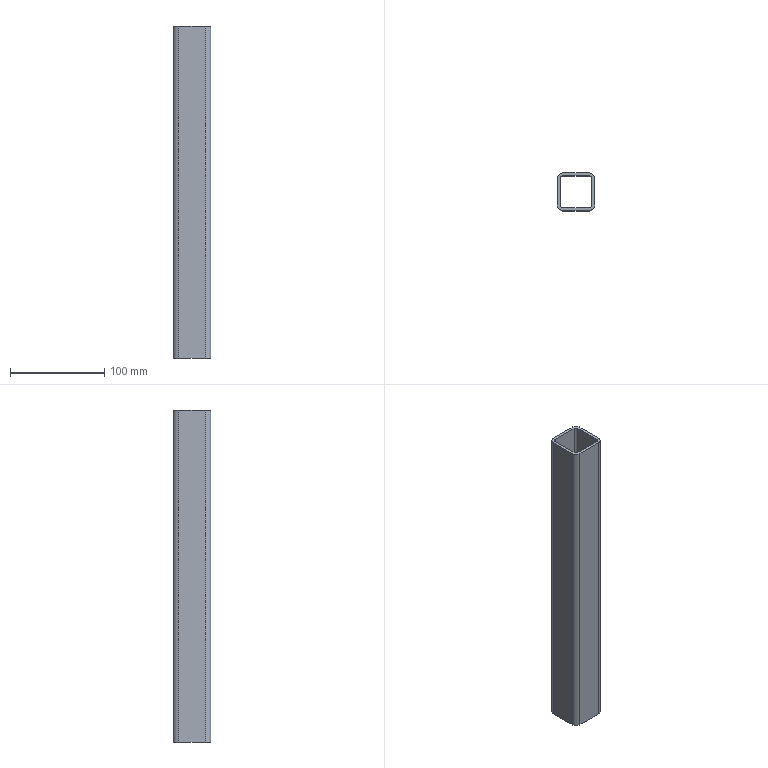Part | STEP file | SN10_003_008-09_TUBO_QUADRADO | 1 solid | 18 faces | box 40 x 40 x 353 mm | volume 148551 mm3 | plane 10 | cylinder 8 | commonest cylinder face diameters 6 x4 12 x4
STEP:
#1=CARTESIAN_POINT('',(0.,0.,0.));
#2=DIRECTION('',(0.,0.,1.));
#3=DIRECTION('',(1.,0.,0.));
#4=AXIS2_PLACEMENT_3D('',#1,#2,#3);
#5=CARTESIAN_POINT('',(3482.,140.,-373.));
#6=VERTEX_POINT('',#5);
#7=CARTESIAN_POINT('',(3488.,146.,-373.));
#8=VERTEX_POINT('',#7);
#9=CARTESIAN_POINT('',(3482.,146.,-373.));
#10=DIRECTION('',(0.,0.,1.));
#11=DIRECTION('',(1.,0.,0.));
#12=AXIS2_PLACEMENT_3D('',#9,#10,#11);
#13=CIRCLE('',#12,6.);
#14=CARTESIAN_POINT('',(3482.,146.,-196.5));
#15=DIRECTION('',(0.,0.,1.));
#16=DIRECTION('',(0.,-1.,0.));
#17=AXIS2_PLACEMENT_3D('',#14,#15,#16);
#18=CYLINDRICAL_SURFACE('',#17,6.);
#19=CARTESIAN_POINT('',(-4.712,-176.5));
#20=DIRECTION('',(1.,0.));
#21=VECTOR('',#20,1.);
#22=LINE('',#19,#21);
#23=(GEOMETRIC_REPRESENTATION_CONTEXT(2)PARAMETRIC_REPRESENTATION_CONTEXT()REPRESENTATION_CONTEXT('',''));
#24=DEFINITIONAL_REPRESENTATION('',(#22),#23);
#25=PCURVE('',#18,#24);
#26=CARTESIAN_POINT('',(0.,0.,-373.));
#27=DIRECTION('',(0.,0.,1.));
#28=DIRECTION('',(1.,0.,0.));
#29=AXIS2_PLACEMENT_3D('',#26,#27,#28);
#30=PLANE('',#29);
#31=CARTESIAN_POINT('',(3482.,146.));
#32=DIRECTION('',(1.,0.));
#33=AXIS2_PLACEMENT_2D('',#31,#32);
#34=CIRCLE('',#33,6.);
#35=(GEOMETRIC_REPRESENTATION_CONTEXT(2)PARAMETRIC_REPRESENTATION_CONTEXT()REPRESENTATION_CONTEXT('',''));
#36=DEFINITIONAL_REPRESENTATION('',(#34),#35);
#37=PCURVE('',#30,#36);
#38=SURFACE_CURVE('',#13,(#25,#37),.PCURVE_S1.);
#39=EDGE_CURVE('',#6,#8,#38,.T.);
#40=ORIENTED_EDGE('',*,*,#39,.T.);
#41=CARTESIAN_POINT('',(3488.,146.,-20.));
#42=VERTEX_POINT('',#41);
#43=CARTESIAN_POINT('',(3488.,146.,-373.));
#44=DIRECTION('',(0.,0.,1.));
#45=VECTOR('',#44,1.);
#46=LINE('',#43,#45);
#47=CARTESIAN_POINT('',(1.571,-176.5));
#48=DIRECTION('',(0.,1.));
#49=VECTOR('',#48,1.);
#50=LINE('',#47,#49);
#51=(GEOMETRIC_REPRESENTATION_CONTEXT(2)PARAMETRIC_REPRESENTATION_CONTEXT()REPRESENTATION_CONTEXT('',''));
#52=DEFINITIONAL_REPRESENTATION('',(#50),#51);
#53=PCURVE('',#18,#52);
#54=CARTESIAN_POINT('',(3488.,146.,-20.));
#55=DIRECTION('',(-1.,0.,0.));
#56=DIRECTION('',(0.,0.,1.));
#57=AXIS2_PLACEMENT_3D('',#54,#55,#56);
#58=PLANE('',#57);
#59=CARTESIAN_POINT('',(-353.,0.));
#60=DIRECTION('',(1.,0.));
#61=VECTOR('',#60,1.);
#62=LINE('',#59,#61);
#63=(GEOMETRIC_REPRESENTATION_CONTEXT(2)PARAMETRIC_REPRESENTATION_CONTEXT()REPRESENTATION_CONTEXT('',''));
#64=DEFINITIONAL_REPRESENTATION('',(#62),#63);
#65=PCURVE('',#58,#64);
#66=SURFACE_CURVE('',#46,(#53,#65),.PCURVE_S1.);
#67=EDGE_CURVE('',#8,#42,#66,.T.);
#68=ORIENTED_EDGE('',*,*,#67,.T.);
#69=CARTESIAN_POINT('',(3482.,140.,-20.));
#70=VERTEX_POINT('',#69);
#71=CARTESIAN_POINT('',(3482.,146.,-20.));
#72=DIRECTION('',(0.,0.,1.));
#73=DIRECTION('',(1.,0.,0.));
#74=AXIS2_PLACEMENT_3D('',#71,#72,#73);
#75=CIRCLE('',#74,6.);
#76=CARTESIAN_POINT('',(-4.712,176.5));
#77=DIRECTION('',(1.,0.));
#78=VECTOR('',#77,1.);
#79=LINE('',#76,#78);
#80=(GEOMETRIC_REPRESENTATION_CONTEXT(2)PARAMETRIC_REPRESENTATION_CONTEXT()REPRESENTATION_CONTEXT('',''));
#81=DEFINITIONAL_REPRESENTATION('',(#79),#80);
#82=PCURVE('',#18,#81);
#83=CARTESIAN_POINT('',(0.,0.,-20.));
#84=DIRECTION('',(0.,0.,1.));
#85=DIRECTION('',(1.,0.,0.));
#86=AXIS2_PLACEMENT_3D('',#83,#84,#85);
#87=PLANE('',#86);
#88=CARTESIAN_POINT('',(3482.,146.));
#89=DIRECTION('',(1.,0.));
#90=AXIS2_PLACEMENT_2D('',#88,#89);
#91=CIRCLE('',#90,6.);
#92=(GEOMETRIC_REPRESENTATION_CONTEXT(2)PARAMETRIC_REPRESENTATION_CONTEXT()REPRESENTATION_CONTEXT('',''));
#93=DEFINITIONAL_REPRESENTATION('',(#91),#92);
#94=PCURVE('',#87,#93);
#95=SURFACE_CURVE('',#75,(#82,#94),.PCURVE_S1.);
#96=EDGE_CURVE('',#70,#42,#95,.T.);
#97=ORIENTED_EDGE('',*,*,#96,.F.);
#98=CARTESIAN_POINT('',(3482.,140.,-373.));
#99=DIRECTION('',(0.,0.,1.));
#100=VECTOR('',#99,1.);
#101=LINE('',#98,#100);
#102=CARTESIAN_POINT('',(0.,-176.5));
#103=DIRECTION('',(0.,1.));
#104=VECTOR('',#103,1.);
#105=LINE('',#102,#104);
#106=(GEOMETRIC_REPRESENTATION_CONTEXT(2)PARAMETRIC_REPRESENTATION_CONTEXT()REPRESENTATION_CONTEXT('',''));
#107=DEFINITIONAL_REPRESENTATION('',(#105),#106);
#108=PCURVE('',#18,#107);
#109=CARTESIAN_POINT('',(3454.,140.,-20.));
#110=DIRECTION('',(0.,1.,0.));
#111=DIRECTION('',(0.,0.,1.));
#112=AXIS2_PLACEMENT_3D('',#109,#110,#111);
#113=PLANE('',#112);
#114=CARTESIAN_POINT('',(-353.,28.));
#115=DIRECTION('',(1.,0.));
#116=VECTOR('',#115,1.);
#117=LINE('',#114,#116);
#118=(GEOMETRIC_REPRESENTATION_CONTEXT(2)PARAMETRIC_REPRESENTATION_CONTEXT()REPRESENTATION_CONTEXT('',''));
#119=DEFINITIONAL_REPRESENTATION('',(#117),#118);
#120=PCURVE('',#113,#119);
#121=SURFACE_CURVE('',#101,(#108,#120),.PCURVE_S1.);
#122=EDGE_CURVE('',#6,#70,#121,.T.);
#123=ORIENTED_EDGE('',*,*,#122,.F.);
#124=EDGE_LOOP('',(#40,#68,#97,#123));
#125=FACE_BOUND('',#124,.T.);
#126=ADVANCED_FACE('',(#125),#18,.T.);
#127=CARTESIAN_POINT('',(3488.,174.,-373.));
#128=VERTEX_POINT('',#127);
#129=CARTESIAN_POINT('',(3488.,146.,-373.));
#130=DIRECTION('',(0.,1.,0.));
#131=VECTOR('',#130,1.);
#132=LINE('',#129,#131);
#133=CARTESIAN_POINT('',(-353.,0.));
#134=DIRECTION('',(0.,1.));
#135=VECTOR('',#134,1.);
#136=LINE('',#133,#135);
#137=(GEOMETRIC_REPRESENTATION_CONTEXT(2)PARAMETRIC_REPRESENTATION_CONTEXT()REPRESENTATION_CONTEXT('',''));
#138=DEFINITIONAL_REPRESENTATION('',(#136),#137);
#139=PCURVE('',#58,#138);
#140=CARTESIAN_POINT('',(3488.,146.));
#141=DIRECTION('',(0.,1.));
#142=VECTOR('',#141,1.);
#143=LINE('',#140,#142);
#144=(GEOMETRIC_REPRESENTATION_CONTEXT(2)PARAMETRIC_REPRESENTATION_CONTEXT()REPRESENTATION_CONTEXT('',''));
#145=DEFINITIONAL_REPRESENTATION('',(#143),#144);
#146=PCURVE('',#30,#145);
#147=SURFACE_CURVE('',#132,(#139,#146),.PCURVE_S1.);
#148=EDGE_CURVE('',#8,#128,#147,.T.);
#149=ORIENTED_EDGE('',*,*,#148,.T.);
#150=CARTESIAN_POINT('',(3488.,174.,-20.));
#151=VERTEX_POINT('',#150);
#152=CARTESIAN_POINT('',(3488.,174.,-20.));
#153=DIRECTION('',(0.,0.,-1.));
#154=VECTOR('',#153,1.);
#155=LINE('',#152,#154);
#156=CARTESIAN_POINT('',(0.,28.));
#157=DIRECTION('',(-1.,0.));
#158=VECTOR('',#157,1.);
#159=LINE('',#156,#158);
#160=(GEOMETRIC_REPRESENTATION_CONTEXT(2)PARAMETRIC_REPRESENTATION_CONTEXT()REPRESENTATION_CONTEXT('',''));
#161=DEFINITIONAL_REPRESENTATION('',(#159),#160);
#162=PCURVE('',#58,#161);
#163=CARTESIAN_POINT('',(3482.,174.,-196.5));
#164=DIRECTION('',(0.,0.,1.));
#165=DIRECTION('',(1.,0.,0.));
#166=AXIS2_PLACEMENT_3D('',#163,#164,#165);
#167=CYLINDRICAL_SURFACE('',#166,6.);
#168=CARTESIAN_POINT('',(0.,176.5));
#169=DIRECTION('',(0.,-1.));
#170=VECTOR('',#169,1.);
#171=LINE('',#168,#170);
#172=(GEOMETRIC_REPRESENTATION_CONTEXT(2)PARAMETRIC_REPRESENTATION_CONTEXT()REPRESENTATION_CONTEXT('',''));
#173=DEFINITIONAL_REPRESENTATION('',(#171),#172);
#174=PCURVE('',#167,#173);
#175=SURFACE_CURVE('',#155,(#162,#174),.PCURVE_S1.);
#176=EDGE_CURVE('',#151,#128,#175,.T.);
#177=ORIENTED_EDGE('',*,*,#176,.F.);
#178=CARTESIAN_POINT('',(3488.,146.,-20.));
#179=DIRECTION('',(0.,1.,0.));
#180=VECTOR('',#179,1.);
#181=LINE('',#178,#180);
#182=CARTESIAN_POINT('',(0.,0.));
#183=DIRECTION('',(0.,1.));
#184=VECTOR('',#183,1.);
#185=LINE('',#182,#184);
#186=(GEOMETRIC_REPRESENTATION_CONTEXT(2)PARAMETRIC_REPRESENTATION_CONTEXT()REPRESENTATION_CONTEXT('',''));
#187=DEFINITIONAL_REPRESENTATION('',(#185),#186);
#188=PCURVE('',#58,#187);
#189=CARTESIAN_POINT('',(3488.,146.));
#190=DIRECTION('',(0.,1.));
#191=VECTOR('',#190,1.);
#192=LINE('',#189,#191);
#193=(GEOMETRIC_REPRESENTATION_CONTEXT(2)PARAMETRIC_REPRESENTATION_CONTEXT()REPRESENTATION_CONTEXT('',''));
#194=DEFINITIONAL_REPRESENTATION('',(#192),#193);
#195=PCURVE('',#87,#194);
#196=SURFACE_CURVE('',#181,(#188,#195),.PCURVE_S1.);
#197=EDGE_CURVE('',#42,#151,#196,.T.);
#198=ORIENTED_EDGE('',*,*,#197,.F.);
#199=ORIENTED_EDGE('',*,*,#67,.F.);
#200=EDGE_LOOP('',(#149,#177,#198,#199));
#201=FACE_BOUND('',#200,.T.);
#202=ADVANCED_FACE('',(#201),#58,.F.);
#203=CARTESIAN_POINT('',(3482.,180.,-373.));
#204=VERTEX_POINT('',#203);
#205=CARTESIAN_POINT('',(3482.,174.,-373.));
#206=DIRECTION('',(0.,0.,1.));
#207=DIRECTION('',(1.,0.,0.));
#208=AXIS2_PLACEMENT_3D('',#205,#206,#207);
#209=CIRCLE('',#208,6.);
#210=CARTESIAN_POINT('',(0.,-176.5));
#211=DIRECTION('',(1.,0.));
#212=VECTOR('',#211,1.);
#213=LINE('',#210,#212);
#214=(GEOMETRIC_REPRESENTATION_CONTEXT(2)PARAMETRIC_REPRESENTATION_CONTEXT()REPRESENTATION_CONTEXT('',''));
#215=DEFINITIONAL_REPRESENTATION('',(#213),#214);
#216=PCURVE('',#167,#215);
#217=CARTESIAN_POINT('',(3482.,174.));
#218=DIRECTION('',(1.,0.));
#219=AXIS2_PLACEMENT_2D('',#217,#218);
#220=CIRCLE('',#219,6.);
#221=(GEOMETRIC_REPRESENTATION_CONTEXT(2)PARAMETRIC_REPRESENTATION_CONTEXT()REPRESENTATION_CONTEXT('',''));
#222=DEFINITIONAL_REPRESENTATION('',(#220),#221);
#223=PCURVE('',#30,#222);
#224=SURFACE_CURVE('',#209,(#216,#223),.PCURVE_S1.);
#225=EDGE_CURVE('',#128,#204,#224,.T.);
#226=ORIENTED_EDGE('',*,*,#225,.T.);
#227=CARTESIAN_POINT('',(3482.,180.,-20.));
#228=VERTEX_POINT('',#227);
#229=CARTESIAN_POINT('',(3482.,180.,-373.));
#230=DIRECTION('',(0.,0.,1.));
#231=VECTOR('',#230,1.);
#232=LINE('',#229,#231);
#233=CARTESIAN_POINT('',(1.571,-176.5));
#234=DIRECTION('',(0.,1.));
#235=VECTOR('',#234,1.);
#236=LINE('',#233,#235);
#237=(GEOMETRIC_REPRESENTATION_CONTEXT(2)PARAMETRIC_REPRESENTATION_CONTEXT()REPRESENTATION_CONTEXT('',''));
#238=DEFINITIONAL_REPRESENTATION('',(#236),#237);
#239=PCURVE('',#167,#238);
#240=CARTESIAN_POINT('',(3482.,180.,-20.));
#241=DIRECTION('',(0.,-1.,0.));
#242=DIRECTION('',(0.,0.,-1.));
#243=AXIS2_PLACEMENT_3D('',#240,#241,#242);
#244=PLANE('',#243);
#245=CARTESIAN_POINT('',(353.,0.));
#246=DIRECTION('',(-1.,0.));
#247=VECTOR('',#246,1.);
#248=LINE('',#245,#247);
#249=(GEOMETRIC_REPRESENTATION_CONTEXT(2)PARAMETRIC_REPRESENTATION_CONTEXT()REPRESENTATION_CONTEXT('',''));
#250=DEFINITIONAL_REPRESENTATION('',(#248),#249);
#251=PCURVE('',#244,#250);
#252=SURFACE_CURVE('',#232,(#239,#251),.PCURVE_S1.);
#253=EDGE_CURVE('',#204,#228,#252,.T.);
#254=ORIENTED_EDGE('',*,*,#253,.T.);
#255=CARTESIAN_POINT('',(3482.,174.,-20.));
#256=DIRECTION('',(0.,0.,1.));
#257=DIRECTION('',(1.,0.,0.));
#258=AXIS2_PLACEMENT_3D('',#255,#256,#257);
#259=CIRCLE('',#258,6.);
#260=CARTESIAN_POINT('',(0.,176.5));
#261=DIRECTION('',(1.,0.));
#262=VECTOR('',#261,1.);
#263=LINE('',#260,#262);
#264=(GEOMETRIC_REPRESENTATION_CONTEXT(2)PARAMETRIC_REPRESENTATION_CONTEXT()REPRESENTATION_CONTEXT('',''));
#265=DEFINITIONAL_REPRESENTATION('',(#263),#264);
#266=PCURVE('',#167,#265);
#267=CARTESIAN_POINT('',(3482.,174.));
#268=DIRECTION('',(1.,0.));
#269=AXIS2_PLACEMENT_2D('',#267,#268);
#270=CIRCLE('',#269,6.);
#271=(GEOMETRIC_REPRESENTATION_CONTEXT(2)PARAMETRIC_REPRESENTATION_CONTEXT()REPRESENTATION_CONTEXT('',''));
#272=DEFINITIONAL_REPRESENTATION('',(#270),#271);
#273=PCURVE('',#87,#272);
#274=SURFACE_CURVE('',#259,(#266,#273),.PCURVE_S1.);
#275=EDGE_CURVE('',#151,#228,#274,.T.);
#276=ORIENTED_EDGE('',*,*,#275,.F.);
#277=ORIENTED_EDGE('',*,*,#176,.T.);
#278=EDGE_LOOP('',(#226,#254,#276,#277));
#279=FACE_BOUND('',#278,.T.);
#280=ADVANCED_FACE('',(#279),#167,.T.);
#281=CARTESIAN_POINT('',(3454.,180.,-373.));
#282=VERTEX_POINT('',#281);
#283=CARTESIAN_POINT('',(3482.,180.,-373.));
#284=DIRECTION('',(-1.,0.,0.));
#285=VECTOR('',#284,1.);
#286=LINE('',#283,#285);
#287=CARTESIAN_POINT('',(353.,0.));
#288=DIRECTION('',(0.,-1.));
#289=VECTOR('',#288,1.);
#290=LINE('',#287,#289);
#291=(GEOMETRIC_REPRESENTATION_CONTEXT(2)PARAMETRIC_REPRESENTATION_CONTEXT()REPRESENTATION_CONTEXT('',''));
#292=DEFINITIONAL_REPRESENTATION('',(#290),#291);
#293=PCURVE('',#244,#292);
#294=CARTESIAN_POINT('',(3482.,180.));
#295=DIRECTION('',(-1.,0.));
#296=VECTOR('',#295,1.);
#297=LINE('',#294,#296);
#298=(GEOMETRIC_REPRESENTATION_CONTEXT(2)PARAMETRIC_REPRESENTATION_CONTEXT()REPRESENTATION_CONTEXT('',''));
#299=DEFINITIONAL_REPRESENTATION('',(#297),#298);
#300=PCURVE('',#30,#299);
#301=SURFACE_CURVE('',#286,(#293,#300),.PCURVE_S1.);
#302=EDGE_CURVE('',#204,#282,#301,.T.);
#303=ORIENTED_EDGE('',*,*,#302,.T.);
#304=CARTESIAN_POINT('',(3454.,180.,-20.));
#305=VERTEX_POINT('',#304);
#306=CARTESIAN_POINT('',(3454.,180.,-20.));
#307=DIRECTION('',(0.,0.,-1.));
#308=VECTOR('',#307,1.);
#309=LINE('',#306,#308);
#310=CARTESIAN_POINT('',(0.,-28.));
#311=DIRECTION('',(1.,0.));
#312=VECTOR('',#311,1.);
#313=LINE('',#310,#312);
#314=(GEOMETRIC_REPRESENTATION_CONTEXT(2)PARAMETRIC_REPRESENTATION_CONTEXT()REPRESENTATION_CONTEXT('',''));
#315=DEFINITIONAL_REPRESENTATION('',(#313),#314);
#316=PCURVE('',#244,#315);
#317=CARTESIAN_POINT('',(3454.,174.,-196.5));
#318=DIRECTION('',(0.,0.,1.));
#319=DIRECTION('',(0.,1.,0.));
#320=AXIS2_PLACEMENT_3D('',#317,#318,#319);
#321=CYLINDRICAL_SURFACE('',#320,6.);
#322=CARTESIAN_POINT('',(0.,176.5));
#323=DIRECTION('',(0.,-1.));
#324=VECTOR('',#323,1.);
#325=LINE('',#322,#324);
#326=(GEOMETRIC_REPRESENTATION_CONTEXT(2)PARAMETRIC_REPRESENTATION_CONTEXT()REPRESENTATION_CONTEXT('',''));
#327=DEFINITIONAL_REPRESENTATION('',(#325),#326);
#328=PCURVE('',#321,#327);
#329=SURFACE_CURVE('',#309,(#316,#328),.PCURVE_S1.);
#330=EDGE_CURVE('',#305,#282,#329,.T.);
#331=ORIENTED_EDGE('',*,*,#330,.F.);
#332=CARTESIAN_POINT('',(3482.,180.,-20.));
#333=DIRECTION('',(-1.,0.,0.));
#334=VECTOR('',#333,1.);
#335=LINE('',#332,#334);
#336=CARTESIAN_POINT('',(0.,0.));
#337=DIRECTION('',(0.,-1.));
#338=VECTOR('',#337,1.);
#339=LINE('',#336,#338);
#340=(GEOMETRIC_REPRESENTATION_CONTEXT(2)PARAMETRIC_REPRESENTATION_CONTEXT()REPRESENTATION_CONTEXT('',''));
#341=DEFINITIONAL_REPRESENTATION('',(#339),#340);
#342=PCURVE('',#244,#341);
#343=CARTESIAN_POINT('',(3482.,180.));
#344=DIRECTION('',(-1.,0.));
#345=VECTOR('',#344,1.);
#346=LINE('',#343,#345);
#347=(GEOMETRIC_REPRESENTATION_CONTEXT(2)PARAMETRIC_REPRESENTATION_CONTEXT()REPRESENTATION_CONTEXT('',''));
#348=DEFINITIONAL_REPRESENTATION('',(#346),#347);
#349=PCURVE('',#87,#348);
#350=SURFACE_CURVE('',#335,(#342,#349),.PCURVE_S1.);
#351=EDGE_CURVE('',#228,#305,#350,.T.);
#352=ORIENTED_EDGE('',*,*,#351,.F.);
#353=ORIENTED_EDGE('',*,*,#253,.F.);
#354=EDGE_LOOP('',(#303,#331,#352,#353));
#355=FACE_BOUND('',#354,.T.);
#356=ADVANCED_FACE('',(#355),#244,.F.);
#357=CARTESIAN_POINT('',(3448.,174.,-373.));
#358=VERTEX_POINT('',#357);
#359=CARTESIAN_POINT('',(3454.,174.,-373.));
#360=DIRECTION('',(0.,0.,1.));
#361=DIRECTION('',(1.,0.,0.));
#362=AXIS2_PLACEMENT_3D('',#359,#360,#361);
#363=CIRCLE('',#362,6.);
#364=CARTESIAN_POINT('',(-1.571,-176.5));
#365=DIRECTION('',(1.,0.));
#366=VECTOR('',#365,1.);
#367=LINE('',#364,#366);
#368=(GEOMETRIC_REPRESENTATION_CONTEXT(2)PARAMETRIC_REPRESENTATION_CONTEXT()REPRESENTATION_CONTEXT('',''));
#369=DEFINITIONAL_REPRESENTATION('',(#367),#368);
#370=PCURVE('',#321,#369);
#371=CARTESIAN_POINT('',(3454.,174.));
#372=DIRECTION('',(1.,0.));
#373=AXIS2_PLACEMENT_2D('',#371,#372);
#374=CIRCLE('',#373,6.);
#375=(GEOMETRIC_REPRESENTATION_CONTEXT(2)PARAMETRIC_REPRESENTATION_CONTEXT()REPRESENTATION_CONTEXT('',''));
#376=DEFINITIONAL_REPRESENTATION('',(#374),#375);
#377=PCURVE('',#30,#376);
#378=SURFACE_CURVE('',#363,(#370,#377),.PCURVE_S1.);
#379=EDGE_CURVE('',#282,#358,#378,.T.);
#380=ORIENTED_EDGE('',*,*,#379,.T.);
#381=CARTESIAN_POINT('',(3448.,174.,-20.));
#382=VERTEX_POINT('',#381);
#383=CARTESIAN_POINT('',(3448.,174.,-373.));
#384=DIRECTION('',(0.,0.,1.));
#385=VECTOR('',#384,1.);
#386=LINE('',#383,#385);
#387=CARTESIAN_POINT('',(1.571,-176.5));
#388=DIRECTION('',(0.,1.));
#389=VECTOR('',#388,1.);
#390=LINE('',#387,#389);
#391=(GEOMETRIC_REPRESENTATION_CONTEXT(2)PARAMETRIC_REPRESENTATION_CONTEXT()REPRESENTATION_CONTEXT('',''));
#392=DEFINITIONAL_REPRESENTATION('',(#390),#391);
#393=PCURVE('',#321,#392);
#394=CARTESIAN_POINT('',(3448.,174.,-20.));
#395=DIRECTION('',(1.,0.,0.));
#396=DIRECTION('',(0.,0.,-1.));
#397=AXIS2_PLACEMENT_3D('',#394,#395,#396);
#398=PLANE('',#397);
#399=CARTESIAN_POINT('',(353.,0.));
#400=DIRECTION('',(-1.,0.));
#401=VECTOR('',#400,1.);
#402=LINE('',#399,#401);
#403=(GEOMETRIC_REPRESENTATION_CONTEXT(2)PARAMETRIC_REPRESENTATION_CONTEXT()REPRESENTATION_CONTEXT('',''));
#404=DEFINITIONAL_REPRESENTATION('',(#402),#403);
#405=PCURVE('',#398,#404);
#406=SURFACE_CURVE('',#386,(#393,#405),.PCURVE_S1.);
#407=EDGE_CURVE('',#358,#382,#406,.T.);
#408=ORIENTED_EDGE('',*,*,#407,.T.);
#409=CARTESIAN_POINT('',(3454.,174.,-20.));
#410=DIRECTION('',(0.,0.,1.));
#411=DIRECTION('',(1.,0.,0.));
#412=AXIS2_PLACEMENT_3D('',#409,#410,#411);
#413=CIRCLE('',#412,6.);
#414=CARTESIAN_POINT('',(-1.571,176.5));
#415=DIRECTION('',(1.,0.));
#416=VECTOR('',#415,1.);
#417=LINE('',#414,#416);
#418=(GEOMETRIC_REPRESENTATION_CONTEXT(2)PARAMETRIC_REPRESENTATION_CONTEXT()REPRESENTATION_CONTEXT('',''));
#419=DEFINITIONAL_REPRESENTATION('',(#417),#418);
#420=PCURVE('',#321,#419);
#421=CARTESIAN_POINT('',(3454.,174.));
#422=DIRECTION('',(1.,0.));
#423=AXIS2_PLACEMENT_2D('',#421,#422);
#424=CIRCLE('',#423,6.);
#425=(GEOMETRIC_REPRESENTATION_CONTEXT(2)PARAMETRIC_REPRESENTATION_CONTEXT()REPRESENTATION_CONTEXT('',''));
#426=DEFINITIONAL_REPRESENTATION('',(#424),#425);
#427=PCURVE('',#87,#426);
#428=SURFACE_CURVE('',#413,(#420,#427),.PCURVE_S1.);
#429=EDGE_CURVE('',#305,#382,#428,.T.);
#430=ORIENTED_EDGE('',*,*,#429,.F.);
#431=ORIENTED_EDGE('',*,*,#330,.T.);
#432=EDGE_LOOP('',(#380,#408,#430,#431));
#433=FACE_BOUND('',#432,.T.);
#434=ADVANCED_FACE('',(#433),#321,.T.);
#435=CARTESIAN_POINT('',(3448.,146.,-373.));
#436=VERTEX_POINT('',#435);
#437=CARTESIAN_POINT('',(3448.,174.,-373.));
#438=DIRECTION('',(0.,-1.,0.));
#439=VECTOR('',#438,1.);
#440=LINE('',#437,#439);
#441=CARTESIAN_POINT('',(353.,0.));
#442=DIRECTION('',(0.,-1.));
#443=VECTOR('',#442,1.);
#444=LINE('',#441,#443);
#445=(GEOMETRIC_REPRESENTATION_CONTEXT(2)PARAMETRIC_REPRESENTATION_CONTEXT()REPRESENTATION_CONTEXT('',''));
#446=DEFINITIONAL_REPRESENTATION('',(#444),#445);
#447=PCURVE('',#398,#446);
#448=CARTESIAN_POINT('',(3448.,174.));
#449=DIRECTION('',(0.,-1.));
#450=VECTOR('',#449,1.);
#451=LINE('',#448,#450);
#452=(GEOMETRIC_REPRESENTATION_CONTEXT(2)PARAMETRIC_REPRESENTATION_CONTEXT()REPRESENTATION_CONTEXT('',''));
#453=DEFINITIONAL_REPRESENTATION('',(#451),#452);
#454=PCURVE('',#30,#453);
#455=SURFACE_CURVE('',#440,(#447,#454),.PCURVE_S1.);
#456=EDGE_CURVE('',#358,#436,#455,.T.);
#457=ORIENTED_EDGE('',*,*,#456,.T.);
#458=CARTESIAN_POINT('',(3448.,146.,-20.));
#459=VERTEX_POINT('',#458);
#460=CARTESIAN_POINT('',(3448.,146.,-20.));
#461=DIRECTION('',(0.,0.,-1.));
#462=VECTOR('',#461,1.);
#463=LINE('',#460,#462);
#464=CARTESIAN_POINT('',(0.,-28.));
#465=DIRECTION('',(1.,0.));
#466=VECTOR('',#465,1.);
#467=LINE('',#464,#466);
#468=(GEOMETRIC_REPRESENTATION_CONTEXT(2)PARAMETRIC_REPRESENTATION_CONTEXT()REPRESENTATION_CONTEXT('',''));
#469=DEFINITIONAL_REPRESENTATION('',(#467),#468);
#470=PCURVE('',#398,#469);
#471=CARTESIAN_POINT('',(3454.,146.,-196.5));
#472=DIRECTION('',(0.,0.,1.));
#473=DIRECTION('',(-1.,0.,0.));
#474=AXIS2_PLACEMENT_3D('',#471,#472,#473);
#475=CYLINDRICAL_SURFACE('',#474,6.);
#476=CARTESIAN_POINT('',(0.,176.5));
#477=DIRECTION('',(0.,-1.));
#478=VECTOR('',#477,1.);
#479=LINE('',#476,#478);
#480=(GEOMETRIC_REPRESENTATION_CONTEXT(2)PARAMETRIC_REPRESENTATION_CONTEXT()REPRESENTATION_CONTEXT('',''));
#481=DEFINITIONAL_REPRESENTATION('',(#479),#480);
#482=PCURVE('',#475,#481);
#483=SURFACE_CURVE('',#463,(#470,#482),.PCURVE_S1.);
#484=EDGE_CURVE('',#459,#436,#483,.T.);
#485=ORIENTED_EDGE('',*,*,#484,.F.);
#486=CARTESIAN_POINT('',(3448.,174.,-20.));
#487=DIRECTION('',(0.,-1.,0.));
#488=VECTOR('',#487,1.);
#489=LINE('',#486,#488);
#490=CARTESIAN_POINT('',(0.,0.));
#491=DIRECTION('',(0.,-1.));
#492=VECTOR('',#491,1.);
#493=LINE('',#490,#492);
#494=(GEOMETRIC_REPRESENTATION_CONTEXT(2)PARAMETRIC_REPRESENTATION_CONTEXT()REPRESENTATION_CONTEXT('',''));
#495=DEFINITIONAL_REPRESENTATION('',(#493),#494);
#496=PCURVE('',#398,#495);
#497=CARTESIAN_POINT('',(3448.,174.));
#498=DIRECTION('',(0.,-1.));
#499=VECTOR('',#498,1.);
#500=LINE('',#497,#499);
#501=(GEOMETRIC_REPRESENTATION_CONTEXT(2)PARAMETRIC_REPRESENTATION_CONTEXT()REPRESENTATION_CONTEXT('',''));
#502=DEFINITIONAL_REPRESENTATION('',(#500),#501);
#503=PCURVE('',#87,#502);
#504=SURFACE_CURVE('',#489,(#496,#503),.PCURVE_S1.);
#505=EDGE_CURVE('',#382,#459,#504,.T.);
#506=ORIENTED_EDGE('',*,*,#505,.F.);
#507=ORIENTED_EDGE('',*,*,#407,.F.);
#508=EDGE_LOOP('',(#457,#485,#506,#507));
#509=FACE_BOUND('',#508,.T.);
#510=ADVANCED_FACE('',(#509),#398,.F.);
#511=CARTESIAN_POINT('',(3454.,140.,-373.));
#512=VERTEX_POINT('',#511);
#513=CARTESIAN_POINT('',(3454.,146.,-373.));
#514=DIRECTION('',(0.,0.,1.));
#515=DIRECTION('',(1.,0.,0.));
#516=AXIS2_PLACEMENT_3D('',#513,#514,#515);
#517=CIRCLE('',#516,6.);
#518=CARTESIAN_POINT('',(-3.142,-176.5));
#519=DIRECTION('',(1.,0.));
#520=VECTOR('',#519,1.);
#521=LINE('',#518,#520);
#522=(GEOMETRIC_REPRESENTATION_CONTEXT(2)PARAMETRIC_REPRESENTATION_CONTEXT()REPRESENTATION_CONTEXT('',''));
#523=DEFINITIONAL_REPRESENTATION('',(#521),#522);
#524=PCURVE('',#475,#523);
#525=CARTESIAN_POINT('',(3454.,146.));
#526=DIRECTION('',(1.,0.));
#527=AXIS2_PLACEMENT_2D('',#525,#526);
#528=CIRCLE('',#527,6.);
#529=(GEOMETRIC_REPRESENTATION_CONTEXT(2)PARAMETRIC_REPRESENTATION_CONTEXT()REPRESENTATION_CONTEXT('',''));
#530=DEFINITIONAL_REPRESENTATION('',(#528),#529);
#531=PCURVE('',#30,#530);
#532=SURFACE_CURVE('',#517,(#524,#531),.PCURVE_S1.);
#533=EDGE_CURVE('',#436,#512,#532,.T.);
#534=ORIENTED_EDGE('',*,*,#533,.T.);
#535=CARTESIAN_POINT('',(3454.,140.,-20.));
#536=VERTEX_POINT('',#535);
#537=CARTESIAN_POINT('',(3454.,140.,-373.));
#538=DIRECTION('',(0.,0.,1.));
#539=VECTOR('',#538,1.);
#540=LINE('',#537,#539);
#541=CARTESIAN_POINT('',(1.571,-176.5));
#542=DIRECTION('',(0.,1.));
#543=VECTOR('',#542,1.);
#544=LINE('',#541,#543);
#545=(GEOMETRIC_REPRESENTATION_CONTEXT(2)PARAMETRIC_REPRESENTATION_CONTEXT()REPRESENTATION_CONTEXT('',''));
#546=DEFINITIONAL_REPRESENTATION('',(#544),#545);
#547=PCURVE('',#475,#546);
#548=CARTESIAN_POINT('',(-353.,0.));
#549=DIRECTION('',(1.,0.));
#550=VECTOR('',#549,1.);
#551=LINE('',#548,#550);
#552=(GEOMETRIC_REPRESENTATION_CONTEXT(2)PARAMETRIC_REPRESENTATION_CONTEXT()REPRESENTATION_CONTEXT('',''));
#553=DEFINITIONAL_REPRESENTATION('',(#551),#552);
#554=PCURVE('',#113,#553);
#555=SURFACE_CURVE('',#540,(#547,#554),.PCURVE_S1.);
#556=EDGE_CURVE('',#512,#536,#555,.T.);
#557=ORIENTED_EDGE('',*,*,#556,.T.);
#558=CARTESIAN_POINT('',(3454.,146.,-20.));
#559=DIRECTION('',(0.,0.,1.));
#560=DIRECTION('',(1.,0.,0.));
#561=AXIS2_PLACEMENT_3D('',#558,#559,#560);
#562=CIRCLE('',#561,6.);
#563=CARTESIAN_POINT('',(-3.142,176.5));
#564=DIRECTION('',(1.,0.));
#565=VECTOR('',#564,1.);
#566=LINE('',#563,#565);
#567=(GEOMETRIC_REPRESENTATION_CONTEXT(2)PARAMETRIC_REPRESENTATION_CONTEXT()REPRESENTATION_CONTEXT('',''));
#568=DEFINITIONAL_REPRESENTATION('',(#566),#567);
#569=PCURVE('',#475,#568);
#570=CARTESIAN_POINT('',(3454.,146.));
#571=DIRECTION('',(1.,0.));
#572=AXIS2_PLACEMENT_2D('',#570,#571);
#573=CIRCLE('',#572,6.);
#574=(GEOMETRIC_REPRESENTATION_CONTEXT(2)PARAMETRIC_REPRESENTATION_CONTEXT()REPRESENTATION_CONTEXT('',''));
#575=DEFINITIONAL_REPRESENTATION('',(#573),#574);
#576=PCURVE('',#87,#575);
#577=SURFACE_CURVE('',#562,(#569,#576),.PCURVE_S1.);
#578=EDGE_CURVE('',#459,#536,#577,.T.);
#579=ORIENTED_EDGE('',*,*,#578,.F.);
#580=ORIENTED_EDGE('',*,*,#484,.T.);
#581=EDGE_LOOP('',(#534,#557,#579,#580));
#582=FACE_BOUND('',#581,.T.);
#583=ADVANCED_FACE('',(#582),#475,.T.);
#584=CARTESIAN_POINT('',(3454.,140.,-373.));
#585=DIRECTION('',(1.,0.,0.));
#586=VECTOR('',#585,1.);
#587=LINE('',#584,#586);
#588=CARTESIAN_POINT('',(-353.,0.));
#589=DIRECTION('',(0.,1.));
#590=VECTOR('',#589,1.);
#591=LINE('',#588,#590);
#592=(GEOMETRIC_REPRESENTATION_CONTEXT(2)PARAMETRIC_REPRESENTATION_CONTEXT()REPRESENTATION_CONTEXT('',''));
#593=DEFINITIONAL_REPRESENTATION('',(#591),#592);
#594=PCURVE('',#113,#593);
#595=CARTESIAN_POINT('',(3454.,140.));
#596=DIRECTION('',(1.,0.));
#597=VECTOR('',#596,1.);
#598=LINE('',#595,#597);
#599=(GEOMETRIC_REPRESENTATION_CONTEXT(2)PARAMETRIC_REPRESENTATION_CONTEXT()REPRESENTATION_CONTEXT('',''));
#600=DEFINITIONAL_REPRESENTATION('',(#598),#599);
#601=PCURVE('',#30,#600);
#602=SURFACE_CURVE('',#587,(#594,#601),.PCURVE_S1.);
#603=EDGE_CURVE('',#512,#6,#602,.T.);
#604=ORIENTED_EDGE('',*,*,#603,.T.);
#605=ORIENTED_EDGE('',*,*,#122,.T.);
#606=CARTESIAN_POINT('',(3454.,140.,-20.));
#607=DIRECTION('',(1.,0.,0.));
#608=VECTOR('',#607,1.);
#609=LINE('',#606,#608);
#610=CARTESIAN_POINT('',(0.,0.));
#611=DIRECTION('',(0.,1.));
#612=VECTOR('',#611,1.);
#613=LINE('',#610,#612);
#614=(GEOMETRIC_REPRESENTATION_CONTEXT(2)PARAMETRIC_REPRESENTATION_CONTEXT()REPRESENTATION_CONTEXT('',''));
#615=DEFINITIONAL_REPRESENTATION('',(#613),#614);
#616=PCURVE('',#113,#615);
#617=CARTESIAN_POINT('',(3454.,140.));
#618=DIRECTION('',(1.,0.));
#619=VECTOR('',#618,1.);
#620=LINE('',#617,#619);
#621=(GEOMETRIC_REPRESENTATION_CONTEXT(2)PARAMETRIC_REPRESENTATION_CONTEXT()REPRESENTATION_CONTEXT('',''));
#622=DEFINITIONAL_REPRESENTATION('',(#620),#621);
#623=PCURVE('',#87,#622);
#624=SURFACE_CURVE('',#609,(#616,#623),.PCURVE_S1.);
#625=EDGE_CURVE('',#536,#70,#624,.T.);
#626=ORIENTED_EDGE('',*,*,#625,.F.);
#627=ORIENTED_EDGE('',*,*,#556,.F.);
#628=EDGE_LOOP('',(#604,#605,#626,#627));
#629=FACE_BOUND('',#628,.T.);
#630=ADVANCED_FACE('',(#629),#113,.F.);
#631=CARTESIAN_POINT('',(3485.,146.,-20.));
#632=VERTEX_POINT('',#631);
#633=CARTESIAN_POINT('',(3485.,146.,-373.));
#634=VERTEX_POINT('',#633);
#635=CARTESIAN_POINT('',(3485.,146.,-20.));
#636=DIRECTION('',(0.,0.,-1.));
#637=VECTOR('',#636,1.);
#638=LINE('',#635,#637);
#639=CARTESIAN_POINT('',(3485.,174.,-20.));
#640=DIRECTION('',(1.,0.,0.));
#641=DIRECTION('',(0.,0.,-1.));
#642=AXIS2_PLACEMENT_3D('',#639,#640,#641);
#643=PLANE('',#642);
#644=CARTESIAN_POINT('',(0.,-28.));
#645=DIRECTION('',(1.,0.));
#646=VECTOR('',#645,1.);
#647=LINE('',#644,#646);
#648=(GEOMETRIC_REPRESENTATION_CONTEXT(2)PARAMETRIC_REPRESENTATION_CONTEXT()REPRESENTATION_CONTEXT('',''));
#649=DEFINITIONAL_REPRESENTATION('',(#647),#648);
#650=PCURVE('',#643,#649);
#651=CARTESIAN_POINT('',(3482.,146.,-196.5));
#652=DIRECTION('',(0.,0.,1.));
#653=DIRECTION('',(0.,-1.,0.));
#654=AXIS2_PLACEMENT_3D('',#651,#652,#653);
#655=CYLINDRICAL_SURFACE('',#654,3.);
#656=CARTESIAN_POINT('',(1.571,176.5));
#657=DIRECTION('',(0.,-1.));
#658=VECTOR('',#657,1.);
#659=LINE('',#656,#658);
#660=(GEOMETRIC_REPRESENTATION_CONTEXT(2)PARAMETRIC_REPRESENTATION_CONTEXT()REPRESENTATION_CONTEXT('',''));
#661=DEFINITIONAL_REPRESENTATION('',(#659),#660);
#662=PCURVE('',#655,#661);
#663=SURFACE_CURVE('',#638,(#650,#662),.PCURVE_S1.);
#664=EDGE_CURVE('',#632,#634,#663,.T.);
#665=ORIENTED_EDGE('',*,*,#664,.F.);
#666=CARTESIAN_POINT('',(3485.,174.,-20.));
#667=VERTEX_POINT('',#666);
#668=CARTESIAN_POINT('',(3485.,174.,-20.));
#669=DIRECTION('',(0.,-1.,0.));
#670=VECTOR('',#669,1.);
#671=LINE('',#668,#670);
#672=CARTESIAN_POINT('',(0.,0.));
#673=DIRECTION('',(0.,-1.));
#674=VECTOR('',#673,1.);
#675=LINE('',#672,#674);
#676=(GEOMETRIC_REPRESENTATION_CONTEXT(2)PARAMETRIC_REPRESENTATION_CONTEXT()REPRESENTATION_CONTEXT('',''));
#677=DEFINITIONAL_REPRESENTATION('',(#675),#676);
#678=PCURVE('',#643,#677);
#679=CARTESIAN_POINT('',(3485.,174.));
#680=DIRECTION('',(0.,-1.));
#681=VECTOR('',#680,1.);
#682=LINE('',#679,#681);
#683=(GEOMETRIC_REPRESENTATION_CONTEXT(2)PARAMETRIC_REPRESENTATION_CONTEXT()REPRESENTATION_CONTEXT('',''));
#684=DEFINITIONAL_REPRESENTATION('',(#682),#683);
#685=PCURVE('',#87,#684);
#686=SURFACE_CURVE('',#671,(#678,#685),.PCURVE_S1.);
#687=EDGE_CURVE('',#667,#632,#686,.T.);
#688=ORIENTED_EDGE('',*,*,#687,.F.);
#689=CARTESIAN_POINT('',(3485.,174.,-373.));
#690=VERTEX_POINT('',#689);
#691=CARTESIAN_POINT('',(3485.,174.,-20.));
#692=DIRECTION('',(0.,0.,-1.));
#693=VECTOR('',#692,1.);
#694=LINE('',#691,#693);
#695=CARTESIAN_POINT('',(0.,0.));
#696=DIRECTION('',(1.,0.));
#697=VECTOR('',#696,1.);
#698=LINE('',#695,#697);
#699=(GEOMETRIC_REPRESENTATION_CONTEXT(2)PARAMETRIC_REPRESENTATION_CONTEXT()REPRESENTATION_CONTEXT('',''));
#700=DEFINITIONAL_REPRESENTATION('',(#698),#699);
#701=PCURVE('',#643,#700);
#702=CARTESIAN_POINT('',(3482.,174.,-196.5));
#703=DIRECTION('',(0.,0.,1.));
#704=DIRECTION('',(1.,0.,0.));
#705=AXIS2_PLACEMENT_3D('',#702,#703,#704);
#706=CYLINDRICAL_SURFACE('',#705,3.);
#707=CARTESIAN_POINT('',(0.,176.5));
#708=DIRECTION('',(0.,-1.));
#709=VECTOR('',#708,1.);
#710=LINE('',#707,#709);
#711=(GEOMETRIC_REPRESENTATION_CONTEXT(2)PARAMETRIC_REPRESENTATION_CONTEXT()REPRESENTATION_CONTEXT('',''));
#712=DEFINITIONAL_REPRESENTATION('',(#710),#711);
#713=PCURVE('',#706,#712);
#714=SURFACE_CURVE('',#694,(#701,#713),.PCURVE_S1.);
#715=EDGE_CURVE('',#667,#690,#714,.T.);
#716=ORIENTED_EDGE('',*,*,#715,.T.);
#717=CARTESIAN_POINT('',(3485.,174.,-373.));
#718=DIRECTION('',(0.,-1.,0.));
#719=VECTOR('',#718,1.);
#720=LINE('',#717,#719);
#721=CARTESIAN_POINT('',(353.,0.));
#722=DIRECTION('',(0.,-1.));
#723=VECTOR('',#722,1.);
#724=LINE('',#721,#723);
#725=(GEOMETRIC_REPRESENTATION_CONTEXT(2)PARAMETRIC_REPRESENTATION_CONTEXT()REPRESENTATION_CONTEXT('',''));
#726=DEFINITIONAL_REPRESENTATION('',(#724),#725);
#727=PCURVE('',#643,#726);
#728=CARTESIAN_POINT('',(3485.,174.));
#729=DIRECTION('',(0.,-1.));
#730=VECTOR('',#729,1.);
#731=LINE('',#728,#730);
#732=(GEOMETRIC_REPRESENTATION_CONTEXT(2)PARAMETRIC_REPRESENTATION_CONTEXT()REPRESENTATION_CONTEXT('',''));
#733=DEFINITIONAL_REPRESENTATION('',(#731),#732);
#734=PCURVE('',#30,#733);
#735=SURFACE_CURVE('',#720,(#727,#734),.PCURVE_S1.);
#736=EDGE_CURVE('',#690,#634,#735,.T.);
#737=ORIENTED_EDGE('',*,*,#736,.T.);
#738=EDGE_LOOP('',(#665,#688,#716,#737));
#739=FACE_BOUND('',#738,.T.);
#740=ADVANCED_FACE('',(#739),#643,.F.);
#741=CARTESIAN_POINT('',(3482.,143.,-373.));
#742=VERTEX_POINT('',#741);
#743=CARTESIAN_POINT('',(3482.,146.,-373.));
#744=DIRECTION('',(0.,0.,1.));
#745=DIRECTION('',(1.,0.,0.));
#746=AXIS2_PLACEMENT_3D('',#743,#744,#745);
#747=CIRCLE('',#746,3.);
#748=CARTESIAN_POINT('',(-4.712,-176.5));
#749=DIRECTION('',(1.,0.));
#750=VECTOR('',#749,1.);
#751=LINE('',#748,#750);
#752=(GEOMETRIC_REPRESENTATION_CONTEXT(2)PARAMETRIC_REPRESENTATION_CONTEXT()REPRESENTATION_CONTEXT('',''));
#753=DEFINITIONAL_REPRESENTATION('',(#751),#752);
#754=PCURVE('',#655,#753);
#755=CARTESIAN_POINT('',(3482.,146.));
#756=DIRECTION('',(1.,0.));
#757=AXIS2_PLACEMENT_2D('',#755,#756);
#758=CIRCLE('',#757,3.);
#759=(GEOMETRIC_REPRESENTATION_CONTEXT(2)PARAMETRIC_REPRESENTATION_CONTEXT()REPRESENTATION_CONTEXT('',''));
#760=DEFINITIONAL_REPRESENTATION('',(#758),#759);
#761=PCURVE('',#30,#760);
#762=SURFACE_CURVE('',#747,(#754,#761),.PCURVE_S1.);
#763=EDGE_CURVE('',#742,#634,#762,.T.);
#764=ORIENTED_EDGE('',*,*,#763,.T.);
#765=ORIENTED_EDGE('',*,*,#664,.F.);
#766=CARTESIAN_POINT('',(3482.,143.,-20.));
#767=VERTEX_POINT('',#766);
#768=CARTESIAN_POINT('',(3482.,146.,-20.));
#769=DIRECTION('',(0.,0.,1.));
#770=DIRECTION('',(1.,0.,0.));
#771=AXIS2_PLACEMENT_3D('',#768,#769,#770);
#772=CIRCLE('',#771,3.);
#773=CARTESIAN_POINT('',(-4.712,176.5));
#774=DIRECTION('',(1.,0.));
#775=VECTOR('',#774,1.);
#776=LINE('',#773,#775);
#777=(GEOMETRIC_REPRESENTATION_CONTEXT(2)PARAMETRIC_REPRESENTATION_CONTEXT()REPRESENTATION_CONTEXT('',''));
#778=DEFINITIONAL_REPRESENTATION('',(#776),#777);
#779=PCURVE('',#655,#778);
#780=CARTESIAN_POINT('',(3482.,146.));
#781=DIRECTION('',(1.,0.));
#782=AXIS2_PLACEMENT_2D('',#780,#781);
#783=CIRCLE('',#782,3.);
#784=(GEOMETRIC_REPRESENTATION_CONTEXT(2)PARAMETRIC_REPRESENTATION_CONTEXT()REPRESENTATION_CONTEXT('',''));
#785=DEFINITIONAL_REPRESENTATION('',(#783),#784);
#786=PCURVE('',#87,#785);
#787=SURFACE_CURVE('',#772,(#779,#786),.PCURVE_S1.);
#788=EDGE_CURVE('',#767,#632,#787,.T.);
#789=ORIENTED_EDGE('',*,*,#788,.F.);
#790=CARTESIAN_POINT('',(3482.,143.,-373.));
#791=DIRECTION('',(0.,0.,1.));
#792=VECTOR('',#791,1.);
#793=LINE('',#790,#792);
#794=CARTESIAN_POINT('',(0.,-176.5));
#795=DIRECTION('',(0.,1.));
#796=VECTOR('',#795,1.);
#797=LINE('',#794,#796);
#798=(GEOMETRIC_REPRESENTATION_CONTEXT(2)PARAMETRIC_REPRESENTATION_CONTEXT()REPRESENTATION_CONTEXT('',''));
#799=DEFINITIONAL_REPRESENTATION('',(#797),#798);
#800=PCURVE('',#655,#799);
#801=CARTESIAN_POINT('',(3482.,143.,-20.));
#802=DIRECTION('',(0.,-1.,0.));
#803=DIRECTION('',(0.,0.,-1.));
#804=AXIS2_PLACEMENT_3D('',#801,#802,#803);
#805=PLANE('',#804);
#806=CARTESIAN_POINT('',(353.,0.));
#807=DIRECTION('',(-1.,0.));
#808=VECTOR('',#807,1.);
#809=LINE('',#806,#808);
#810=(GEOMETRIC_REPRESENTATION_CONTEXT(2)PARAMETRIC_REPRESENTATION_CONTEXT()REPRESENTATION_CONTEXT('',''));
#811=DEFINITIONAL_REPRESENTATION('',(#809),#810);
#812=PCURVE('',#805,#811);
#813=SURFACE_CURVE('',#793,(#800,#812),.PCURVE_S1.);
#814=EDGE_CURVE('',#742,#767,#813,.T.);
#815=ORIENTED_EDGE('',*,*,#814,.F.);
#816=EDGE_LOOP('',(#764,#765,#789,#815));
#817=FACE_BOUND('',#816,.F.);
#818=ADVANCED_FACE('',(#817),#655,.F.);
#819=CARTESIAN_POINT('',(3454.,143.,-20.));
#820=VERTEX_POINT('',#819);
#821=CARTESIAN_POINT('',(3454.,143.,-373.));
#822=VERTEX_POINT('',#821);
#823=CARTESIAN_POINT('',(3454.,143.,-20.));
#824=DIRECTION('',(0.,0.,-1.));
#825=VECTOR('',#824,1.);
#826=LINE('',#823,#825);
#827=CARTESIAN_POINT('',(0.,-28.));
#828=DIRECTION('',(1.,0.));
#829=VECTOR('',#828,1.);
#830=LINE('',#827,#829);
#831=(GEOMETRIC_REPRESENTATION_CONTEXT(2)PARAMETRIC_REPRESENTATION_CONTEXT()REPRESENTATION_CONTEXT('',''));
#832=DEFINITIONAL_REPRESENTATION('',(#830),#831);
#833=PCURVE('',#805,#832);
#834=CARTESIAN_POINT('',(3454.,146.,-196.5));
#835=DIRECTION('',(0.,0.,1.));
#836=DIRECTION('',(-1.,0.,0.));
#837=AXIS2_PLACEMENT_3D('',#834,#835,#836);
#838=CYLINDRICAL_SURFACE('',#837,3.);
#839=CARTESIAN_POINT('',(1.571,176.5));
#840=DIRECTION('',(0.,-1.));
#841=VECTOR('',#840,1.);
#842=LINE('',#839,#841);
#843=(GEOMETRIC_REPRESENTATION_CONTEXT(2)PARAMETRIC_REPRESENTATION_CONTEXT()REPRESENTATION_CONTEXT('',''));
#844=DEFINITIONAL_REPRESENTATION('',(#842),#843);
#845=PCURVE('',#838,#844);
#846=SURFACE_CURVE('',#826,(#833,#845),.PCURVE_S1.);
#847=EDGE_CURVE('',#820,#822,#846,.T.);
#848=ORIENTED_EDGE('',*,*,#847,.F.);
#849=CARTESIAN_POINT('',(3482.,143.,-20.));
#850=DIRECTION('',(-1.,0.,0.));
#851=VECTOR('',#850,1.);
#852=LINE('',#849,#851);
#853=CARTESIAN_POINT('',(0.,0.));
#854=DIRECTION('',(0.,-1.));
#855=VECTOR('',#854,1.);
#856=LINE('',#853,#855);
#857=(GEOMETRIC_REPRESENTATION_CONTEXT(2)PARAMETRIC_REPRESENTATION_CONTEXT()REPRESENTATION_CONTEXT('',''));
#858=DEFINITIONAL_REPRESENTATION('',(#856),#857);
#859=PCURVE('',#805,#858);
#860=CARTESIAN_POINT('',(3482.,143.));
#861=DIRECTION('',(-1.,0.));
#862=VECTOR('',#861,1.);
#863=LINE('',#860,#862);
#864=(GEOMETRIC_REPRESENTATION_CONTEXT(2)PARAMETRIC_REPRESENTATION_CONTEXT()REPRESENTATION_CONTEXT('',''));
#865=DEFINITIONAL_REPRESENTATION('',(#863),#864);
#866=PCURVE('',#87,#865);
#867=SURFACE_CURVE('',#852,(#859,#866),.PCURVE_S1.);
#868=EDGE_CURVE('',#767,#820,#867,.T.);
#869=ORIENTED_EDGE('',*,*,#868,.F.);
#870=ORIENTED_EDGE('',*,*,#814,.F.);
#871=CARTESIAN_POINT('',(3482.,143.,-373.));
#872=DIRECTION('',(-1.,0.,0.));
#873=VECTOR('',#872,1.);
#874=LINE('',#871,#873);
#875=CARTESIAN_POINT('',(353.,0.));
#876=DIRECTION('',(0.,-1.));
#877=VECTOR('',#876,1.);
#878=LINE('',#875,#877);
#879=(GEOMETRIC_REPRESENTATION_CONTEXT(2)PARAMETRIC_REPRESENTATION_CONTEXT()REPRESENTATION_CONTEXT('',''));
#880=DEFINITIONAL_REPRESENTATION('',(#878),#879);
#881=PCURVE('',#805,#880);
#882=CARTESIAN_POINT('',(3482.,143.));
#883=DIRECTION('',(-1.,0.));
#884=VECTOR('',#883,1.);
#885=LINE('',#882,#884);
#886=(GEOMETRIC_REPRESENTATION_CONTEXT(2)PARAMETRIC_REPRESENTATION_CONTEXT()REPRESENTATION_CONTEXT('',''));
#887=DEFINITIONAL_REPRESENTATION('',(#885),#886);
#888=PCURVE('',#30,#887);
#889=SURFACE_CURVE('',#874,(#881,#888),.PCURVE_S1.);
#890=EDGE_CURVE('',#742,#822,#889,.T.);
#891=ORIENTED_EDGE('',*,*,#890,.T.);
#892=EDGE_LOOP('',(#848,#869,#870,#891));
#893=FACE_BOUND('',#892,.T.);
#894=ADVANCED_FACE('',(#893),#805,.F.);
#895=CARTESIAN_POINT('',(3451.,146.,-373.));
#896=VERTEX_POINT('',#895);
#897=CARTESIAN_POINT('',(3454.,146.,-373.));
#898=DIRECTION('',(0.,0.,1.));
#899=DIRECTION('',(1.,0.,0.));
#900=AXIS2_PLACEMENT_3D('',#897,#898,#899);
#901=CIRCLE('',#900,3.);
#902=CARTESIAN_POINT('',(-3.142,-176.5));
#903=DIRECTION('',(1.,0.));
#904=VECTOR('',#903,1.);
#905=LINE('',#902,#904);
#906=(GEOMETRIC_REPRESENTATION_CONTEXT(2)PARAMETRIC_REPRESENTATION_CONTEXT()REPRESENTATION_CONTEXT('',''));
#907=DEFINITIONAL_REPRESENTATION('',(#905),#906);
#908=PCURVE('',#838,#907);
#909=CARTESIAN_POINT('',(3454.,146.));
#910=DIRECTION('',(1.,0.));
#911=AXIS2_PLACEMENT_2D('',#909,#910);
#912=CIRCLE('',#911,3.);
#913=(GEOMETRIC_REPRESENTATION_CONTEXT(2)PARAMETRIC_REPRESENTATION_CONTEXT()REPRESENTATION_CONTEXT('',''));
#914=DEFINITIONAL_REPRESENTATION('',(#912),#913);
#915=PCURVE('',#30,#914);
#916=SURFACE_CURVE('',#901,(#908,#915),.PCURVE_S1.);
#917=EDGE_CURVE('',#896,#822,#916,.T.);
#918=ORIENTED_EDGE('',*,*,#917,.T.);
#919=ORIENTED_EDGE('',*,*,#847,.F.);
#920=CARTESIAN_POINT('',(3451.,146.,-20.));
#921=VERTEX_POINT('',#920);
#922=CARTESIAN_POINT('',(3454.,146.,-20.));
#923=DIRECTION('',(0.,0.,1.));
#924=DIRECTION('',(1.,0.,0.));
#925=AXIS2_PLACEMENT_3D('',#922,#923,#924);
#926=CIRCLE('',#925,3.);
#927=CARTESIAN_POINT('',(-3.142,176.5));
#928=DIRECTION('',(1.,0.));
#929=VECTOR('',#928,1.);
#930=LINE('',#927,#929);
#931=(GEOMETRIC_REPRESENTATION_CONTEXT(2)PARAMETRIC_REPRESENTATION_CONTEXT()REPRESENTATION_CONTEXT('',''));
#932=DEFINITIONAL_REPRESENTATION('',(#930),#931);
#933=PCURVE('',#838,#932);
#934=CARTESIAN_POINT('',(3454.,146.));
#935=DIRECTION('',(1.,0.));
#936=AXIS2_PLACEMENT_2D('',#934,#935);
#937=CIRCLE('',#936,3.);
#938=(GEOMETRIC_REPRESENTATION_CONTEXT(2)PARAMETRIC_REPRESENTATION_CONTEXT()REPRESENTATION_CONTEXT('',''));
#939=DEFINITIONAL_REPRESENTATION('',(#937),#938);
#940=PCURVE('',#87,#939);
#941=SURFACE_CURVE('',#926,(#933,#940),.PCURVE_S1.);
#942=EDGE_CURVE('',#921,#820,#941,.T.);
#943=ORIENTED_EDGE('',*,*,#942,.F.);
#944=CARTESIAN_POINT('',(3451.,146.,-373.));
#945=DIRECTION('',(0.,0.,1.));
#946=VECTOR('',#945,1.);
#947=LINE('',#944,#946);
#948=CARTESIAN_POINT('',(0.,-176.5));
#949=DIRECTION('',(0.,1.));
#950=VECTOR('',#949,1.);
#951=LINE('',#948,#950);
#952=(GEOMETRIC_REPRESENTATION_CONTEXT(2)PARAMETRIC_REPRESENTATION_CONTEXT()REPRESENTATION_CONTEXT('',''));
#953=DEFINITIONAL_REPRESENTATION('',(#951),#952);
#954=PCURVE('',#838,#953);
#955=CARTESIAN_POINT('',(3451.,146.,-20.));
#956=DIRECTION('',(-1.,0.,0.));
#957=DIRECTION('',(0.,0.,1.));
#958=AXIS2_PLACEMENT_3D('',#955,#956,#957);
#959=PLANE('',#958);
#960=CARTESIAN_POINT('',(-353.,0.));
#961=DIRECTION('',(1.,0.));
#962=VECTOR('',#961,1.);
#963=LINE('',#960,#962);
#964=(GEOMETRIC_REPRESENTATION_CONTEXT(2)PARAMETRIC_REPRESENTATION_CONTEXT()REPRESENTATION_CONTEXT('',''));
#965=DEFINITIONAL_REPRESENTATION('',(#963),#964);
#966=PCURVE('',#959,#965);
#967=SURFACE_CURVE('',#947,(#954,#966),.PCURVE_S1.);
#968=EDGE_CURVE('',#896,#921,#967,.T.);
#969=ORIENTED_EDGE('',*,*,#968,.F.);
#970=EDGE_LOOP('',(#918,#919,#943,#969));
#971=FACE_BOUND('',#970,.F.);
#972=ADVANCED_FACE('',(#971),#838,.F.);
#973=CARTESIAN_POINT('',(3451.,174.,-20.));
#974=VERTEX_POINT('',#973);
#975=CARTESIAN_POINT('',(3451.,174.,-373.));
#976=VERTEX_POINT('',#975);
#977=CARTESIAN_POINT('',(3451.,174.,-20.));
#978=DIRECTION('',(0.,0.,-1.));
#979=VECTOR('',#978,1.);
#980=LINE('',#977,#979);
#981=CARTESIAN_POINT('',(0.,28.));
#982=DIRECTION('',(-1.,0.));
#983=VECTOR('',#982,1.);
#984=LINE('',#981,#983);
#985=(GEOMETRIC_REPRESENTATION_CONTEXT(2)PARAMETRIC_REPRESENTATION_CONTEXT()REPRESENTATION_CONTEXT('',''));
#986=DEFINITIONAL_REPRESENTATION('',(#984),#985);
#987=PCURVE('',#959,#986);
#988=CARTESIAN_POINT('',(3454.,174.,-196.5));
#989=DIRECTION('',(0.,0.,1.));
#990=DIRECTION('',(0.,1.,0.));
#991=AXIS2_PLACEMENT_3D('',#988,#989,#990);
#992=CYLINDRICAL_SURFACE('',#991,3.);
#993=CARTESIAN_POINT('',(1.571,176.5));
#994=DIRECTION('',(0.,-1.));
#995=VECTOR('',#994,1.);
#996=LINE('',#993,#995);
#997=(GEOMETRIC_REPRESENTATION_CONTEXT(2)PARAMETRIC_REPRESENTATION_CONTEXT()REPRESENTATION_CONTEXT('',''));
#998=DEFINITIONAL_REPRESENTATION('',(#996),#997);
#999=PCURVE('',#992,#998);
#1000=SURFACE_CURVE('',#980,(#987,#999),.PCURVE_S1.);
#1001=EDGE_CURVE('',#974,#976,#1000,.T.);
#1002=ORIENTED_EDGE('',*,*,#1001,.F.);
#1003=CARTESIAN_POINT('',(3451.,146.,-20.));
#1004=DIRECTION('',(0.,1.,0.));
#1005=VECTOR('',#1004,1.);
#1006=LINE('',#1003,#1005);
#1007=CARTESIAN_POINT('',(0.,0.));
#1008=DIRECTION('',(0.,1.));
#1009=VECTOR('',#1008,1.);
#1010=LINE('',#1007,#1009);
#1011=(GEOMETRIC_REPRESENTATION_CONTEXT(2)PARAMETRIC_REPRESENTATION_CONTEXT()REPRESENTATION_CONTEXT('',''));
#1012=DEFINITIONAL_REPRESENTATION('',(#1010),#1011);
#1013=PCURVE('',#959,#1012);
#1014=CARTESIAN_POINT('',(3451.,146.));
#1015=DIRECTION('',(0.,1.));
#1016=VECTOR('',#1015,1.);
#1017=LINE('',#1014,#1016);
#1018=(GEOMETRIC_REPRESENTATION_CONTEXT(2)PARAMETRIC_REPRESENTATION_CONTEXT()REPRESENTATION_CONTEXT('',''));
#1019=DEFINITIONAL_REPRESENTATION('',(#1017),#1018);
#1020=PCURVE('',#87,#1019);
#1021=SURFACE_CURVE('',#1006,(#1013,#1020),.PCURVE_S1.);
#1022=EDGE_CURVE('',#921,#974,#1021,.T.);
#1023=ORIENTED_EDGE('',*,*,#1022,.F.);
#1024=ORIENTED_EDGE('',*,*,#968,.F.);
#1025=CARTESIAN_POINT('',(3451.,146.,-373.));
#1026=DIRECTION('',(0.,1.,0.));
#1027=VECTOR('',#1026,1.);
#1028=LINE('',#1025,#1027);
#1029=CARTESIAN_POINT('',(-353.,0.));
#1030=DIRECTION('',(0.,1.));
#1031=VECTOR('',#1030,1.);
#1032=LINE('',#1029,#1031);
#1033=(GEOMETRIC_REPRESENTATION_CONTEXT(2)PARAMETRIC_REPRESENTATION_CONTEXT()REPRESENTATION_CONTEXT('',''));
#1034=DEFINITIONAL_REPRESENTATION('',(#1032),#1033);
#1035=PCURVE('',#959,#1034);
#1036=CARTESIAN_POINT('',(3451.,146.));
#1037=DIRECTION('',(0.,1.));
#1038=VECTOR('',#1037,1.);
#1039=LINE('',#1036,#1038);
#1040=(GEOMETRIC_REPRESENTATION_CONTEXT(2)PARAMETRIC_REPRESENTATION_CONTEXT()REPRESENTATION_CONTEXT('',''));
#1041=DEFINITIONAL_REPRESENTATION('',(#1039),#1040);
#1042=PCURVE('',#30,#1041);
#1043=SURFACE_CURVE('',#1028,(#1035,#1042),.PCURVE_S1.);
#1044=EDGE_CURVE('',#896,#976,#1043,.T.);
#1045=ORIENTED_EDGE('',*,*,#1044,.T.);
#1046=EDGE_LOOP('',(#1002,#1023,#1024,#1045));
#1047=FACE_BOUND('',#1046,.T.);
#1048=ADVANCED_FACE('',(#1047),#959,.F.);
#1049=CARTESIAN_POINT('',(3454.,177.,-373.));
#1050=VERTEX_POINT('',#1049);
#1051=CARTESIAN_POINT('',(3454.,174.,-373.));
#1052=DIRECTION('',(0.,0.,1.));
#1053=DIRECTION('',(1.,0.,0.));
#1054=AXIS2_PLACEMENT_3D('',#1051,#1052,#1053);
#1055=CIRCLE('',#1054,3.);
#1056=CARTESIAN_POINT('',(-1.571,-176.5));
#1057=DIRECTION('',(1.,0.));
#1058=VECTOR('',#1057,1.);
#1059=LINE('',#1056,#1058);
#1060=(GEOMETRIC_REPRESENTATION_CONTEXT(2)PARAMETRIC_REPRESENTATION_CONTEXT()REPRESENTATION_CONTEXT('',''));
#1061=DEFINITIONAL_REPRESENTATION('',(#1059),#1060);
#1062=PCURVE('',#992,#1061);
#1063=CARTESIAN_POINT('',(3454.,174.));
#1064=DIRECTION('',(1.,0.));
#1065=AXIS2_PLACEMENT_2D('',#1063,#1064);
#1066=CIRCLE('',#1065,3.);
#1067=(GEOMETRIC_REPRESENTATION_CONTEXT(2)PARAMETRIC_REPRESENTATION_CONTEXT()REPRESENTATION_CONTEXT('',''));
#1068=DEFINITIONAL_REPRESENTATION('',(#1066),#1067);
#1069=PCURVE('',#30,#1068);
#1070=SURFACE_CURVE('',#1055,(#1062,#1069),.PCURVE_S1.);
#1071=EDGE_CURVE('',#1050,#976,#1070,.T.);
#1072=ORIENTED_EDGE('',*,*,#1071,.T.);
#1073=ORIENTED_EDGE('',*,*,#1001,.F.);
#1074=CARTESIAN_POINT('',(3454.,177.,-20.));
#1075=VERTEX_POINT('',#1074);
#1076=CARTESIAN_POINT('',(3454.,174.,-20.));
#1077=DIRECTION('',(0.,0.,1.));
#1078=DIRECTION('',(1.,0.,0.));
#1079=AXIS2_PLACEMENT_3D('',#1076,#1077,#1078);
#1080=CIRCLE('',#1079,3.);
#1081=CARTESIAN_POINT('',(-1.571,176.5));
#1082=DIRECTION('',(1.,0.));
#1083=VECTOR('',#1082,1.);
#1084=LINE('',#1081,#1083);
#1085=(GEOMETRIC_REPRESENTATION_CONTEXT(2)PARAMETRIC_REPRESENTATION_CONTEXT()REPRESENTATION_CONTEXT('',''));
#1086=DEFINITIONAL_REPRESENTATION('',(#1084),#1085);
#1087=PCURVE('',#992,#1086);
#1088=CARTESIAN_POINT('',(3454.,174.));
#1089=DIRECTION('',(1.,0.));
#1090=AXIS2_PLACEMENT_2D('',#1088,#1089);
#1091=CIRCLE('',#1090,3.);
#1092=(GEOMETRIC_REPRESENTATION_CONTEXT(2)PARAMETRIC_REPRESENTATION_CONTEXT()REPRESENTATION_CONTEXT('',''));
#1093=DEFINITIONAL_REPRESENTATION('',(#1091),#1092);
#1094=PCURVE('',#87,#1093);
#1095=SURFACE_CURVE('',#1080,(#1087,#1094),.PCURVE_S1.);
#1096=EDGE_CURVE('',#1075,#974,#1095,.T.);
#1097=ORIENTED_EDGE('',*,*,#1096,.F.);
#1098=CARTESIAN_POINT('',(3454.,177.,-373.));
#1099=DIRECTION('',(0.,0.,1.));
#1100=VECTOR('',#1099,1.);
#1101=LINE('',#1098,#1100);
#1102=CARTESIAN_POINT('',(0.,-176.5));
#1103=DIRECTION('',(0.,1.));
#1104=VECTOR('',#1103,1.);
#1105=LINE('',#1102,#1104);
#1106=(GEOMETRIC_REPRESENTATION_CONTEXT(2)PARAMETRIC_REPRESENTATION_CONTEXT()REPRESENTATION_CONTEXT('',''));
#1107=DEFINITIONAL_REPRESENTATION('',(#1105),#1106);
#1108=PCURVE('',#992,#1107);
#1109=CARTESIAN_POINT('',(3454.,177.,-20.));
#1110=DIRECTION('',(0.,1.,0.));
#1111=DIRECTION('',(0.,0.,1.));
#1112=AXIS2_PLACEMENT_3D('',#1109,#1110,#1111);
#1113=PLANE('',#1112);
#1114=CARTESIAN_POINT('',(-353.,0.));
#1115=DIRECTION('',(1.,0.));
#1116=VECTOR('',#1115,1.);
#1117=LINE('',#1114,#1116);
#1118=(GEOMETRIC_REPRESENTATION_CONTEXT(2)PARAMETRIC_REPRESENTATION_CONTEXT()REPRESENTATION_CONTEXT('',''));
#1119=DEFINITIONAL_REPRESENTATION('',(#1117),#1118);
#1120=PCURVE('',#1113,#1119);
#1121=SURFACE_CURVE('',#1101,(#1108,#1120),.PCURVE_S1.);
#1122=EDGE_CURVE('',#1050,#1075,#1121,.T.);
#1123=ORIENTED_EDGE('',*,*,#1122,.F.);
#1124=EDGE_LOOP('',(#1072,#1073,#1097,#1123));
#1125=FACE_BOUND('',#1124,.F.);
#1126=ADVANCED_FACE('',(#1125),#992,.F.);
#1127=CARTESIAN_POINT('',(3482.,177.,-20.));
#1128=VERTEX_POINT('',#1127);
#1129=CARTESIAN_POINT('',(3482.,177.,-373.));
#1130=VERTEX_POINT('',#1129);
#1131=CARTESIAN_POINT('',(3482.,177.,-20.));
#1132=DIRECTION('',(0.,0.,-1.));
#1133=VECTOR('',#1132,1.);
#1134=LINE('',#1131,#1133);
#1135=CARTESIAN_POINT('',(0.,28.));
#1136=DIRECTION('',(-1.,0.));
#1137=VECTOR('',#1136,1.);
#1138=LINE('',#1135,#1137);
#1139=(GEOMETRIC_REPRESENTATION_CONTEXT(2)PARAMETRIC_REPRESENTATION_CONTEXT()REPRESENTATION_CONTEXT('',''));
#1140=DEFINITIONAL_REPRESENTATION('',(#1138),#1139);
#1141=PCURVE('',#1113,#1140);
#1142=CARTESIAN_POINT('',(1.571,176.5));
#1143=DIRECTION('',(0.,-1.));
#1144=VECTOR('',#1143,1.);
#1145=LINE('',#1142,#1144);
#1146=(GEOMETRIC_REPRESENTATION_CONTEXT(2)PARAMETRIC_REPRESENTATION_CONTEXT()REPRESENTATION_CONTEXT('',''));
#1147=DEFINITIONAL_REPRESENTATION('',(#1145),#1146);
#1148=PCURVE('',#706,#1147);
#1149=SURFACE_CURVE('',#1134,(#1141,#1148),.PCURVE_S1.);
#1150=EDGE_CURVE('',#1128,#1130,#1149,.T.);
#1151=ORIENTED_EDGE('',*,*,#1150,.F.);
#1152=CARTESIAN_POINT('',(3454.,177.,-20.));
#1153=DIRECTION('',(1.,0.,0.));
#1154=VECTOR('',#1153,1.);
#1155=LINE('',#1152,#1154);
#1156=CARTESIAN_POINT('',(0.,0.));
#1157=DIRECTION('',(0.,1.));
#1158=VECTOR('',#1157,1.);
#1159=LINE('',#1156,#1158);
#1160=(GEOMETRIC_REPRESENTATION_CONTEXT(2)PARAMETRIC_REPRESENTATION_CONTEXT()REPRESENTATION_CONTEXT('',''));
#1161=DEFINITIONAL_REPRESENTATION('',(#1159),#1160);
#1162=PCURVE('',#1113,#1161);
#1163=CARTESIAN_POINT('',(3454.,177.));
#1164=DIRECTION('',(1.,0.));
#1165=VECTOR('',#1164,1.);
#1166=LINE('',#1163,#1165);
#1167=(GEOMETRIC_REPRESENTATION_CONTEXT(2)PARAMETRIC_REPRESENTATION_CONTEXT()REPRESENTATION_CONTEXT('',''));
#1168=DEFINITIONAL_REPRESENTATION('',(#1166),#1167);
#1169=PCURVE('',#87,#1168);
#1170=SURFACE_CURVE('',#1155,(#1162,#1169),.PCURVE_S1.);
#1171=EDGE_CURVE('',#1075,#1128,#1170,.T.);
#1172=ORIENTED_EDGE('',*,*,#1171,.F.);
#1173=ORIENTED_EDGE('',*,*,#1122,.F.);
#1174=CARTESIAN_POINT('',(3454.,177.,-373.));
#1175=DIRECTION('',(1.,0.,0.));
#1176=VECTOR('',#1175,1.);
#1177=LINE('',#1174,#1176);
#1178=CARTESIAN_POINT('',(-353.,0.));
#1179=DIRECTION('',(0.,1.));
#1180=VECTOR('',#1179,1.);
#1181=LINE('',#1178,#1180);
#1182=(GEOMETRIC_REPRESENTATION_CONTEXT(2)PARAMETRIC_REPRESENTATION_CONTEXT()REPRESENTATION_CONTEXT('',''));
#1183=DEFINITIONAL_REPRESENTATION('',(#1181),#1182);
#1184=PCURVE('',#1113,#1183);
#1185=CARTESIAN_POINT('',(3454.,177.));
#1186=DIRECTION('',(1.,0.));
#1187=VECTOR('',#1186,1.);
#1188=LINE('',#1185,#1187);
#1189=(GEOMETRIC_REPRESENTATION_CONTEXT(2)PARAMETRIC_REPRESENTATION_CONTEXT()REPRESENTATION_CONTEXT('',''));
#1190=DEFINITIONAL_REPRESENTATION('',(#1188),#1189);
#1191=PCURVE('',#30,#1190);
#1192=SURFACE_CURVE('',#1177,(#1184,#1191),.PCURVE_S1.);
#1193=EDGE_CURVE('',#1050,#1130,#1192,.T.);
#1194=ORIENTED_EDGE('',*,*,#1193,.T.);
#1195=EDGE_LOOP('',(#1151,#1172,#1173,#1194));
#1196=FACE_BOUND('',#1195,.T.);
#1197=ADVANCED_FACE('',(#1196),#1113,.F.);
#1198=CARTESIAN_POINT('',(3482.,174.,-373.));
#1199=DIRECTION('',(0.,0.,1.));
#1200=DIRECTION('',(1.,0.,0.));
#1201=AXIS2_PLACEMENT_3D('',#1198,#1199,#1200);
#1202=CIRCLE('',#1201,3.);
#1203=CARTESIAN_POINT('',(0.,-176.5));
#1204=DIRECTION('',(1.,0.));
#1205=VECTOR('',#1204,1.);
#1206=LINE('',#1203,#1205);
#1207=(GEOMETRIC_REPRESENTATION_CONTEXT(2)PARAMETRIC_REPRESENTATION_CONTEXT()REPRESENTATION_CONTEXT('',''));
#1208=DEFINITIONAL_REPRESENTATION('',(#1206),#1207);
#1209=PCURVE('',#706,#1208);
#1210=CARTESIAN_POINT('',(3482.,174.));
#1211=DIRECTION('',(1.,0.));
#1212=AXIS2_PLACEMENT_2D('',#1210,#1211);
#1213=CIRCLE('',#1212,3.);
#1214=(GEOMETRIC_REPRESENTATION_CONTEXT(2)PARAMETRIC_REPRESENTATION_CONTEXT()REPRESENTATION_CONTEXT('',''));
#1215=DEFINITIONAL_REPRESENTATION('',(#1213),#1214);
#1216=PCURVE('',#30,#1215);
#1217=SURFACE_CURVE('',#1202,(#1209,#1216),.PCURVE_S1.);
#1218=EDGE_CURVE('',#690,#1130,#1217,.T.);
#1219=ORIENTED_EDGE('',*,*,#1218,.T.);
#1220=ORIENTED_EDGE('',*,*,#1150,.F.);
#1221=CARTESIAN_POINT('',(3482.,174.,-20.));
#1222=DIRECTION('',(0.,0.,1.));
#1223=DIRECTION('',(1.,0.,0.));
#1224=AXIS2_PLACEMENT_3D('',#1221,#1222,#1223);
#1225=CIRCLE('',#1224,3.);
#1226=CARTESIAN_POINT('',(0.,176.5));
#1227=DIRECTION('',(1.,0.));
#1228=VECTOR('',#1227,1.);
#1229=LINE('',#1226,#1228);
#1230=(GEOMETRIC_REPRESENTATION_CONTEXT(2)PARAMETRIC_REPRESENTATION_CONTEXT()REPRESENTATION_CONTEXT('',''));
#1231=DEFINITIONAL_REPRESENTATION('',(#1229),#1230);
#1232=PCURVE('',#706,#1231);
#1233=CARTESIAN_POINT('',(3482.,174.));
#1234=DIRECTION('',(1.,0.));
#1235=AXIS2_PLACEMENT_2D('',#1233,#1234);
#1236=CIRCLE('',#1235,3.);
#1237=(GEOMETRIC_REPRESENTATION_CONTEXT(2)PARAMETRIC_REPRESENTATION_CONTEXT()REPRESENTATION_CONTEXT('',''));
#1238=DEFINITIONAL_REPRESENTATION('',(#1236),#1237);
#1239=PCURVE('',#87,#1238);
#1240=SURFACE_CURVE('',#1225,(#1232,#1239),.PCURVE_S1.);
#1241=EDGE_CURVE('',#667,#1128,#1240,.T.);
#1242=ORIENTED_EDGE('',*,*,#1241,.F.);
#1243=ORIENTED_EDGE('',*,*,#715,.T.);
#1244=EDGE_LOOP('',(#1219,#1220,#1242,#1243));
#1245=FACE_BOUND('',#1244,.F.);
#1246=ADVANCED_FACE('',(#1245),#706,.F.);
#1247=ORIENTED_EDGE('',*,*,#96,.T.);
#1248=ORIENTED_EDGE('',*,*,#197,.T.);
#1249=ORIENTED_EDGE('',*,*,#275,.T.);
#1250=ORIENTED_EDGE('',*,*,#351,.T.);
#1251=ORIENTED_EDGE('',*,*,#429,.T.);
#1252=ORIENTED_EDGE('',*,*,#505,.T.);
#1253=ORIENTED_EDGE('',*,*,#578,.T.);
#1254=ORIENTED_EDGE('',*,*,#625,.T.);
#1255=EDGE_LOOP('',(#1247,#1248,#1249,#1250,#1251,#1252,#1253,#1254));
#1256=FACE_BOUND('',#1255,.T.);
#1257=ORIENTED_EDGE('',*,*,#687,.T.);
#1258=ORIENTED_EDGE('',*,*,#788,.F.);
#1259=ORIENTED_EDGE('',*,*,#868,.T.);
#1260=ORIENTED_EDGE('',*,*,#942,.F.);
#1261=ORIENTED_EDGE('',*,*,#1022,.T.);
#1262=ORIENTED_EDGE('',*,*,#1096,.F.);
#1263=ORIENTED_EDGE('',*,*,#1171,.T.);
#1264=ORIENTED_EDGE('',*,*,#1241,.F.);
#1265=EDGE_LOOP('',(#1257,#1258,#1259,#1260,#1261,#1262,#1263,#1264));
#1266=FACE_BOUND('',#1265,.T.);
#1267=ADVANCED_FACE('',(#1256,#1266),#87,.T.);
#1268=ORIENTED_EDGE('',*,*,#603,.F.);
#1269=ORIENTED_EDGE('',*,*,#533,.F.);
#1270=ORIENTED_EDGE('',*,*,#456,.F.);
#1271=ORIENTED_EDGE('',*,*,#379,.F.);
#1272=ORIENTED_EDGE('',*,*,#302,.F.);
#1273=ORIENTED_EDGE('',*,*,#225,.F.);
#1274=ORIENTED_EDGE('',*,*,#148,.F.);
#1275=ORIENTED_EDGE('',*,*,#39,.F.);
#1276=EDGE_LOOP('',(#1268,#1269,#1270,#1271,#1272,#1273,#1274,#1275));
#1277=FACE_BOUND('',#1276,.T.);
#1278=ORIENTED_EDGE('',*,*,#1218,.T.);
#1279=ORIENTED_EDGE('',*,*,#1193,.F.);
#1280=ORIENTED_EDGE('',*,*,#1071,.T.);
#1281=ORIENTED_EDGE('',*,*,#1044,.F.);
#1282=ORIENTED_EDGE('',*,*,#917,.T.);
#1283=ORIENTED_EDGE('',*,*,#890,.F.);
#1284=ORIENTED_EDGE('',*,*,#763,.T.);
#1285=ORIENTED_EDGE('',*,*,#736,.F.);
#1286=EDGE_LOOP('',(#1278,#1279,#1280,#1281,#1282,#1283,#1284,#1285));
#1287=FACE_BOUND('',#1286,.T.);
#1288=ADVANCED_FACE('',(#1277,#1287),#30,.F.);
#1289=CLOSED_SHELL('',(#126,#202,#280,#356,#434,#510,#583,#630,#740,#818,#894,#972,#1048,#1126,#1197,#1246,#1267,#1288));
#1290=MANIFOLD_SOLID_BREP('',#1289);
#1291=(LENGTH_UNIT()NAMED_UNIT(*)SI_UNIT(.MILLI.,.METRE.));
#1292=UNCERTAINTY_MEASURE_WITH_UNIT(LENGTH_MEASURE(0.0000001),#1291,'','');
#1293=(NAMED_UNIT(*)PLANE_ANGLE_UNIT()SI_UNIT($,.RADIAN.));
#1294=(NAMED_UNIT(*)SI_UNIT($,.STERADIAN.)SOLID_ANGLE_UNIT());
#1295=(GEOMETRIC_REPRESENTATION_CONTEXT(3)GLOBAL_UNCERTAINTY_ASSIGNED_CONTEXT((#1292))GLOBAL_UNIT_ASSIGNED_CONTEXT((#1291,#1293,#1294))REPRESENTATION_CONTEXT('',''));
#1296=ADVANCED_BREP_SHAPE_REPRESENTATION('',(#4,#1290),#1295);